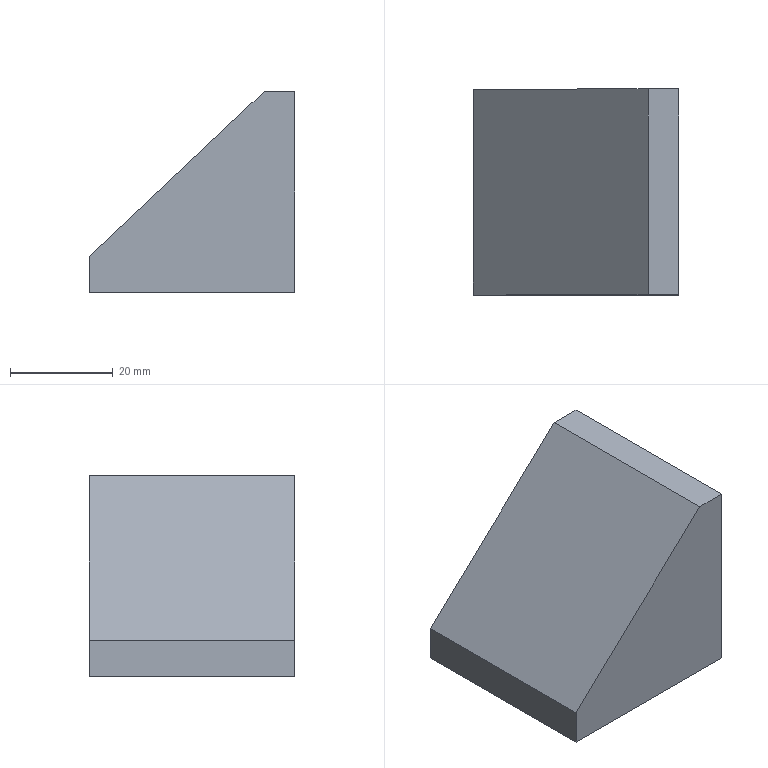Part | SolidWorks | features Extrusion 1, ICE 1 | 1 solid | 10 faces | box 40 x 40 x 39 mm | volume 38929 mm3 | plane 8 | cylinder 2 | commonest cylinder face diameters 33 x2
STEP:
#1=CARTESIAN_POINT('',(38.,20.,36.));
#2=VERTEX_POINT('',#1);
#3=CARTESIAN_POINT('',(38.,20.,3.));
#4=VERTEX_POINT('',#3);
#5=CARTESIAN_POINT('',(38.,20.,19.5));
#6=DIRECTION('',(1.,0.,0.));
#7=DIRECTION('',(0.,0.,-1.));
#8=AXIS2_PLACEMENT_3D('',#5,#6,#7);
#9=CIRCLE('',#8,16.5);
#10=EDGE_CURVE('',#2,#4,#9,.T.);
#11=ORIENTED_EDGE('',*,*,#10,.F.);
#12=CARTESIAN_POINT('',(40.,20.,36.));
#13=VERTEX_POINT('',#12);
#14=CARTESIAN_POINT('',(38.,20.,36.));
#15=DIRECTION('',(1.,0.,0.));
#16=VECTOR('',#15,1000.);
#17=LINE('',#14,#16);
#18=EDGE_CURVE('',#2,#13,#17,.T.);
#19=ORIENTED_EDGE('',*,*,#18,.T.);
#20=CARTESIAN_POINT('',(40.,20.,3.));
#21=VERTEX_POINT('',#20);
#22=CARTESIAN_POINT('',(40.,20.,19.5));
#23=DIRECTION('',(1.,0.,0.));
#24=DIRECTION('',(0.,0.,-1.));
#25=AXIS2_PLACEMENT_3D('',#22,#23,#24);
#26=CIRCLE('',#25,16.5);
#27=EDGE_CURVE('',#13,#21,#26,.T.);
#28=ORIENTED_EDGE('',*,*,#27,.T.);
#29=CARTESIAN_POINT('',(38.,20.,3.));
#30=DIRECTION('',(1.,0.,0.));
#31=VECTOR('',#30,1000.);
#32=LINE('',#29,#31);
#33=EDGE_CURVE('',#4,#21,#32,.T.);
#34=ORIENTED_EDGE('',*,*,#33,.F.);
#35=EDGE_LOOP('',(#11,#19,#28,#34));
#36=FACE_OUTER_BOUND('',#35,.T.);
#37=CARTESIAN_POINT('',(38.,20.,19.5));
#38=DIRECTION('',(1.,0.,0.));
#39=DIRECTION('',(0.,0.,-1.));
#40=AXIS2_PLACEMENT_3D('',#37,#38,#39);
#41=CYLINDRICAL_SURFACE('',#40,16.5);
#42=ADVANCED_FACE('',(#36),#41,.F.);
#43=CARTESIAN_POINT('',(0.,0.,0.));
#44=VERTEX_POINT('',#43);
#45=CARTESIAN_POINT('',(0.,0.,7.));
#46=VERTEX_POINT('',#45);
#47=CARTESIAN_POINT('',(0.,0.,7.));
#48=DIRECTION('',(0.,0.,1.));
#49=VECTOR('',#48,1000.);
#50=LINE('',#47,#49);
#51=EDGE_CURVE('',#44,#46,#50,.T.);
#52=ORIENTED_EDGE('',*,*,#51,.T.);
#53=CARTESIAN_POINT('',(0.,40.,7.));
#54=VERTEX_POINT('',#53);
#55=CARTESIAN_POINT('',(0.,40.,7.));
#56=DIRECTION('',(0.,-1.,0.));
#57=VECTOR('',#56,1000.);
#58=LINE('',#55,#57);
#59=EDGE_CURVE('',#54,#46,#58,.T.);
#60=ORIENTED_EDGE('',*,*,#59,.F.);
#61=CARTESIAN_POINT('',(0.,40.,0.));
#62=VERTEX_POINT('',#61);
#63=CARTESIAN_POINT('',(0.,40.,7.));
#64=DIRECTION('',(0.,0.,1.));
#65=VECTOR('',#64,1000.);
#66=LINE('',#63,#65);
#67=EDGE_CURVE('',#62,#54,#66,.T.);
#68=ORIENTED_EDGE('',*,*,#67,.F.);
#69=CARTESIAN_POINT('',(0.,40.,0.));
#70=DIRECTION('',(0.,-1.,0.));
#71=VECTOR('',#70,1000.);
#72=LINE('',#69,#71);
#73=EDGE_CURVE('',#62,#44,#72,.T.);
#74=ORIENTED_EDGE('',*,*,#73,.T.);
#75=EDGE_LOOP('',(#52,#60,#68,#74));
#76=FACE_OUTER_BOUND('',#75,.T.);
#77=CARTESIAN_POINT('',(0.,40.,7.));
#78=DIRECTION('',(1.,0.,0.));
#79=DIRECTION('',(0.,0.,-1.));
#80=AXIS2_PLACEMENT_3D('',#77,#78,#79);
#81=PLANE('',#80);
#82=ADVANCED_FACE('',(#76),#81,.F.);
#83=CARTESIAN_POINT('',(34.,0.,39.));
#84=VERTEX_POINT('',#83);
#85=CARTESIAN_POINT('',(34.,0.,39.));
#86=DIRECTION('',(0.7282,0.,0.6854));
#87=VECTOR('',#86,1000.);
#88=LINE('',#85,#87);
#89=EDGE_CURVE('',#46,#84,#88,.T.);
#90=ORIENTED_EDGE('',*,*,#89,.T.);
#91=CARTESIAN_POINT('',(34.,40.,39.));
#92=VERTEX_POINT('',#91);
#93=CARTESIAN_POINT('',(34.,40.,39.));
#94=DIRECTION('',(0.,-1.,0.));
#95=VECTOR('',#94,1000.);
#96=LINE('',#93,#95);
#97=EDGE_CURVE('',#92,#84,#96,.T.);
#98=ORIENTED_EDGE('',*,*,#97,.F.);
#99=CARTESIAN_POINT('',(34.,40.,39.));
#100=DIRECTION('',(0.7282,0.,0.6854));
#101=VECTOR('',#100,1000.);
#102=LINE('',#99,#101);
#103=EDGE_CURVE('',#54,#92,#102,.T.);
#104=ORIENTED_EDGE('',*,*,#103,.F.);
#105=ORIENTED_EDGE('',*,*,#59,.T.);
#106=EDGE_LOOP('',(#90,#98,#104,#105));
#107=FACE_OUTER_BOUND('',#106,.T.);
#108=CARTESIAN_POINT('',(34.,40.,39.));
#109=DIRECTION('',(0.6854,0.,-0.7282));
#110=DIRECTION('',(-0.7282,0.,-0.6854));
#111=AXIS2_PLACEMENT_3D('',#108,#109,#110);
#112=PLANE('',#111);
#113=ADVANCED_FACE('',(#107),#112,.F.);
#114=CARTESIAN_POINT('',(40.,0.,39.));
#115=VERTEX_POINT('',#114);
#116=CARTESIAN_POINT('',(40.,0.,39.));
#117=DIRECTION('',(1.,0.,0.));
#118=VECTOR('',#117,1000.);
#119=LINE('',#116,#118);
#120=EDGE_CURVE('',#84,#115,#119,.T.);
#121=ORIENTED_EDGE('',*,*,#120,.T.);
#122=CARTESIAN_POINT('',(40.,40.,39.));
#123=VERTEX_POINT('',#122);
#124=CARTESIAN_POINT('',(40.,40.,39.));
#125=DIRECTION('',(0.,-1.,0.));
#126=VECTOR('',#125,1000.);
#127=LINE('',#124,#126);
#128=EDGE_CURVE('',#123,#115,#127,.T.);
#129=ORIENTED_EDGE('',*,*,#128,.F.);
#130=CARTESIAN_POINT('',(40.,40.,39.));
#131=DIRECTION('',(1.,0.,0.));
#132=VECTOR('',#131,1000.);
#133=LINE('',#130,#132);
#134=EDGE_CURVE('',#92,#123,#133,.T.);
#135=ORIENTED_EDGE('',*,*,#134,.F.);
#136=ORIENTED_EDGE('',*,*,#97,.T.);
#137=EDGE_LOOP('',(#121,#129,#135,#136));
#138=FACE_OUTER_BOUND('',#137,.T.);
#139=CARTESIAN_POINT('',(40.,40.,39.));
#140=DIRECTION('',(0.,0.,-1.));
#141=DIRECTION('',(-1.,0.,0.));
#142=AXIS2_PLACEMENT_3D('',#139,#140,#141);
#143=PLANE('',#142);
#144=ADVANCED_FACE('',(#138),#143,.F.);
#145=CARTESIAN_POINT('',(40.,20.,19.5));
#146=DIRECTION('',(1.,0.,0.));
#147=DIRECTION('',(0.,0.,-1.));
#148=AXIS2_PLACEMENT_3D('',#145,#146,#147);
#149=CIRCLE('',#148,16.5);
#150=EDGE_CURVE('',#21,#13,#149,.T.);
#151=ORIENTED_EDGE('',*,*,#150,.F.);
#152=ORIENTED_EDGE('',*,*,#27,.F.);
#153=EDGE_LOOP('',(#151,#152));
#154=FACE_BOUND('',#153,.T.);
#155=CARTESIAN_POINT('',(40.,0.,0.));
#156=VERTEX_POINT('',#155);
#157=CARTESIAN_POINT('',(40.,0.,0.));
#158=DIRECTION('',(0.,0.,-1.));
#159=VECTOR('',#158,1000.);
#160=LINE('',#157,#159);
#161=EDGE_CURVE('',#115,#156,#160,.T.);
#162=ORIENTED_EDGE('',*,*,#161,.T.);
#163=CARTESIAN_POINT('',(40.,40.,0.));
#164=VERTEX_POINT('',#163);
#165=CARTESIAN_POINT('',(40.,40.,0.));
#166=DIRECTION('',(0.,-1.,0.));
#167=VECTOR('',#166,1000.);
#168=LINE('',#165,#167);
#169=EDGE_CURVE('',#164,#156,#168,.T.);
#170=ORIENTED_EDGE('',*,*,#169,.F.);
#171=CARTESIAN_POINT('',(40.,40.,0.));
#172=DIRECTION('',(0.,0.,-1.));
#173=VECTOR('',#172,1000.);
#174=LINE('',#171,#173);
#175=EDGE_CURVE('',#123,#164,#174,.T.);
#176=ORIENTED_EDGE('',*,*,#175,.F.);
#177=ORIENTED_EDGE('',*,*,#128,.T.);
#178=EDGE_LOOP('',(#162,#170,#176,#177));
#179=FACE_OUTER_BOUND('',#178,.T.);
#180=CARTESIAN_POINT('',(40.,40.,0.));
#181=DIRECTION('',(-1.,0.,0.));
#182=DIRECTION('',(0.,0.,1.));
#183=AXIS2_PLACEMENT_3D('',#180,#181,#182);
#184=PLANE('',#183);
#185=ADVANCED_FACE('',(#154,#179),#184,.F.);
#186=CARTESIAN_POINT('',(0.,0.,0.));
#187=DIRECTION('',(-1.,0.,0.));
#188=VECTOR('',#187,1000.);
#189=LINE('',#186,#188);
#190=EDGE_CURVE('',#156,#44,#189,.T.);
#191=ORIENTED_EDGE('',*,*,#190,.T.);
#192=ORIENTED_EDGE('',*,*,#73,.F.);
#193=CARTESIAN_POINT('',(0.,40.,0.));
#194=DIRECTION('',(-1.,0.,0.));
#195=VECTOR('',#194,1000.);
#196=LINE('',#193,#195);
#197=EDGE_CURVE('',#164,#62,#196,.T.);
#198=ORIENTED_EDGE('',*,*,#197,.F.);
#199=ORIENTED_EDGE('',*,*,#169,.T.);
#200=EDGE_LOOP('',(#191,#192,#198,#199));
#201=FACE_OUTER_BOUND('',#200,.T.);
#202=CARTESIAN_POINT('',(0.,40.,0.));
#203=DIRECTION('',(0.,0.,1.));
#204=DIRECTION('',(1.,0.,0.));
#205=AXIS2_PLACEMENT_3D('',#202,#203,#204);
#206=PLANE('',#205);
#207=ADVANCED_FACE('',(#201),#206,.F.);
#208=ORIENTED_EDGE('',*,*,#67,.T.);
#209=ORIENTED_EDGE('',*,*,#103,.T.);
#210=ORIENTED_EDGE('',*,*,#134,.T.);
#211=ORIENTED_EDGE('',*,*,#175,.T.);
#212=ORIENTED_EDGE('',*,*,#197,.T.);
#213=EDGE_LOOP('',(#208,#209,#210,#211,#212));
#214=FACE_OUTER_BOUND('',#213,.T.);
#215=CARTESIAN_POINT('',(0.,40.,0.));
#216=DIRECTION('',(0.,-1.,0.));
#217=DIRECTION('',(0.,0.,-1.));
#218=AXIS2_PLACEMENT_3D('',#215,#216,#217);
#219=PLANE('',#218);
#220=ADVANCED_FACE('',(#214),#219,.F.);
#221=ORIENTED_EDGE('',*,*,#51,.F.);
#222=ORIENTED_EDGE('',*,*,#190,.F.);
#223=ORIENTED_EDGE('',*,*,#161,.F.);
#224=ORIENTED_EDGE('',*,*,#120,.F.);
#225=ORIENTED_EDGE('',*,*,#89,.F.);
#226=EDGE_LOOP('',(#221,#222,#223,#224,#225));
#227=FACE_OUTER_BOUND('',#226,.T.);
#228=CARTESIAN_POINT('',(0.,0.,0.));
#229=DIRECTION('',(0.,-1.,0.));
#230=DIRECTION('',(0.,0.,-1.));
#231=AXIS2_PLACEMENT_3D('',#228,#229,#230);
#232=PLANE('',#231);
#233=ADVANCED_FACE('',(#227),#232,.T.);
#234=ORIENTED_EDGE('',*,*,#18,.F.);
#235=CARTESIAN_POINT('',(38.,20.,19.5));
#236=DIRECTION('',(1.,0.,0.));
#237=DIRECTION('',(0.,0.,-1.));
#238=AXIS2_PLACEMENT_3D('',#235,#236,#237);
#239=CIRCLE('',#238,16.5);
#240=EDGE_CURVE('',#4,#2,#239,.T.);
#241=ORIENTED_EDGE('',*,*,#240,.F.);
#242=ORIENTED_EDGE('',*,*,#33,.T.);
#243=ORIENTED_EDGE('',*,*,#150,.T.);
#244=EDGE_LOOP('',(#234,#241,#242,#243));
#245=FACE_OUTER_BOUND('',#244,.T.);
#246=CARTESIAN_POINT('',(38.,20.,19.5));
#247=DIRECTION('',(1.,0.,0.));
#248=DIRECTION('',(0.,0.,-1.));
#249=AXIS2_PLACEMENT_3D('',#246,#247,#248);
#250=CYLINDRICAL_SURFACE('',#249,16.5);
#251=ADVANCED_FACE('',(#245),#250,.F.);
#252=ORIENTED_EDGE('',*,*,#240,.T.);
#253=ORIENTED_EDGE('',*,*,#10,.T.);
#254=EDGE_LOOP('',(#252,#253));
#255=FACE_OUTER_BOUND('',#254,.T.);
#256=CARTESIAN_POINT('',(38.,20.,19.5));
#257=DIRECTION('',(1.,0.,0.));
#258=DIRECTION('',(0.,0.,-1.));
#259=AXIS2_PLACEMENT_3D('',#256,#257,#258);
#260=PLANE('',#259);
#261=ADVANCED_FACE('',(#255),#260,.T.);
#262=CLOSED_SHELL('',(#42,#82,#113,#144,#185,#207,#220,#233,#251,#261));
#263=MANIFOLD_SOLID_BREP('',#262);
#264=CARTESIAN_POINT('',(0.,0.,0.));
#265=DIRECTION('',(0.,0.,1.));
#266=DIRECTION('',(1.,0.,0.));
#267=AXIS2_PLACEMENT_3D('',#264,#265,#266);
#268=(LENGTH_UNIT()NAMED_UNIT(*)SI_UNIT(.MILLI.,.METRE.));
#269=UNCERTAINTY_MEASURE_WITH_UNIT(LENGTH_MEASURE(0.00001),#268,'','');
#270=(NAMED_UNIT(*)PLANE_ANGLE_UNIT()SI_UNIT($,.RADIAN.));
#271=(NAMED_UNIT(*)SI_UNIT($,.STERADIAN.)SOLID_ANGLE_UNIT());
#272=(GEOMETRIC_REPRESENTATION_CONTEXT(3)GLOBAL_UNCERTAINTY_ASSIGNED_CONTEXT((#269))GLOBAL_UNIT_ASSIGNED_CONTEXT((#268,#270,#271))REPRESENTATION_CONTEXT('',''));
#273=ADVANCED_BREP_SHAPE_REPRESENTATION('',(#263,#267),#272);